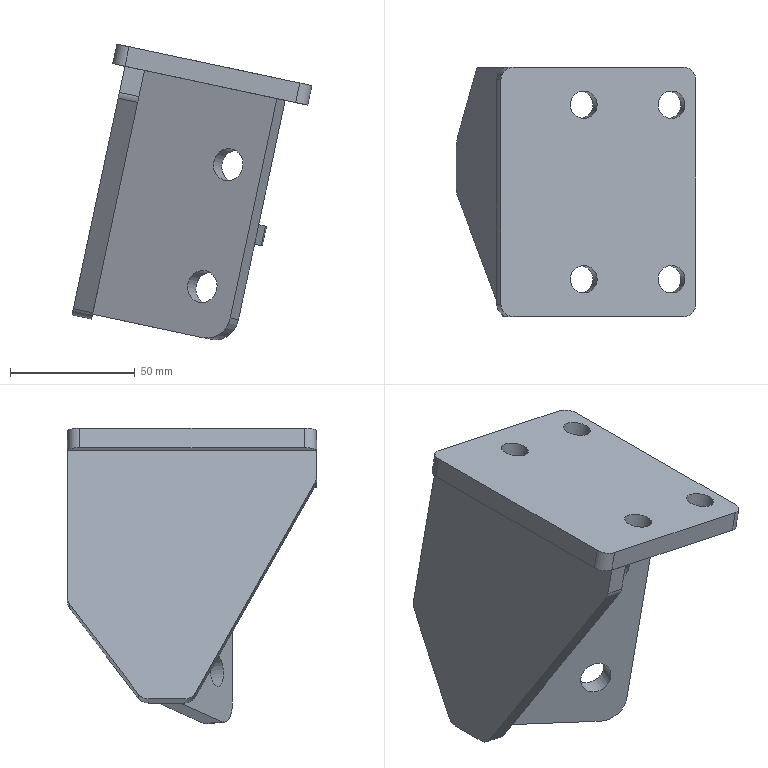Part | STEP file | HL4GZ-1.862.062 (anti-wrap blade seat) | 4 solids | 44 faces | box 96.231 x 100 x 118.639 mm | volume 177743 mm3 | plane 27 | cylinder 17 | commonest cylinder face diameters 10 x10 11 x4 13 x2 20 x1